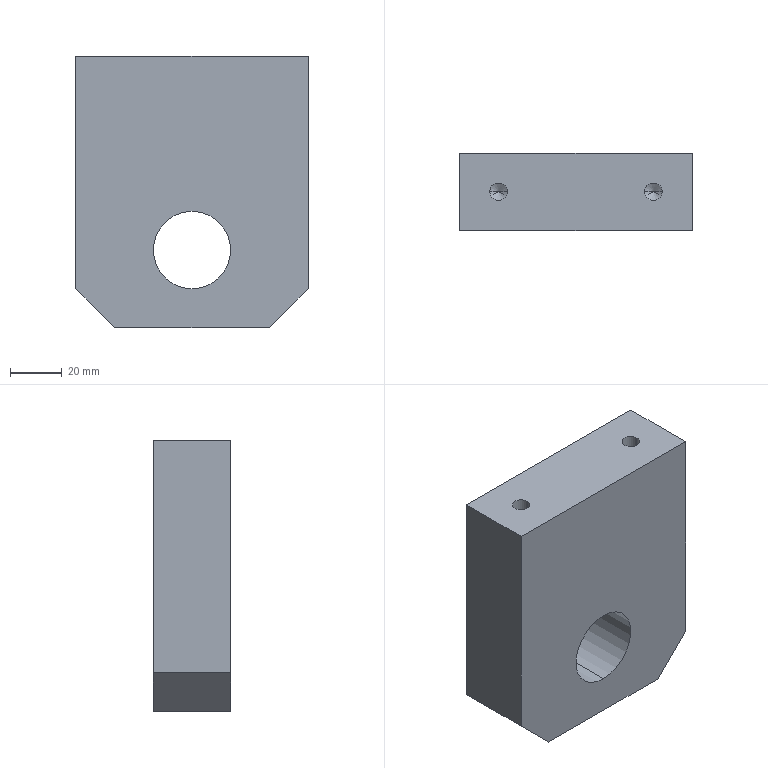Part | STEP file | PN_0020_default | 1 solid | 18 faces | box 90 x 30 x 105 mm | volume 254060 mm3 | plane 8 | cylinder 6 | cone 4 | commonest cylinder face diameters 6.8 x4 30 x2
STEP:
#1=CARTESIAN_POINT('',(0.,0.,0.));
#2=DIRECTION('',(0.,0.,1.));
#3=DIRECTION('',(1.,0.,0.));
#4=AXIS2_PLACEMENT_3D('',#1,#2,#3);
#5=CARTESIAN_POINT('',(-26.6,0.,32.75));
#6=VERTEX_POINT('',#5);
#7=CARTESIAN_POINT('',(-26.6,0.,52.5));
#8=VERTEX_POINT('',#7);
#9=CARTESIAN_POINT('',(-26.6,0.,52.5));
#10=DIRECTION('',(0.,0.,1.));
#11=VECTOR('',#10,1.);
#12=LINE('',#9,#11);
#13=CARTESIAN_POINT('',(-30.,0.,52.5));
#14=DIRECTION('',(0.,0.,1.));
#15=DIRECTION('',(1.,0.,0.));
#16=AXIS2_PLACEMENT_3D('',#13,#14,#15);
#17=CYLINDRICAL_SURFACE('',#16,3.4);
#18=CARTESIAN_POINT('',(6.283,0.));
#19=DIRECTION('',(0.,1.));
#20=VECTOR('',#19,1.);
#21=LINE('',#18,#20);
#22=(GEOMETRIC_REPRESENTATION_CONTEXT(2)PARAMETRIC_REPRESENTATION_CONTEXT()REPRESENTATION_CONTEXT('',''));
#23=DEFINITIONAL_REPRESENTATION('',(#21),#22);
#24=PCURVE('',#17,#23);
#25=CARTESIAN_POINT('',(-30.,0.,52.5));
#26=DIRECTION('',(0.,0.,1.));
#27=DIRECTION('',(1.,0.,0.));
#28=AXIS2_PLACEMENT_3D('',#25,#26,#27);
#29=CYLINDRICAL_SURFACE('',#28,3.4);
#30=CARTESIAN_POINT('',(0.,0.));
#31=DIRECTION('',(0.,1.));
#32=VECTOR('',#31,1.);
#33=LINE('',#30,#32);
#34=(GEOMETRIC_REPRESENTATION_CONTEXT(2)PARAMETRIC_REPRESENTATION_CONTEXT()REPRESENTATION_CONTEXT('',''));
#35=DEFINITIONAL_REPRESENTATION('',(#33),#34);
#36=PCURVE('',#29,#35);
#37=SURFACE_CURVE('',#12,(#24,#36),.PCURVE_S1.);
#38=EDGE_CURVE('',#6,#8,#37,.T.);
#39=ORIENTED_EDGE('',*,*,#38,.T.);
#40=CARTESIAN_POINT('',(-33.4,0.,52.5));
#41=VERTEX_POINT('',#40);
#42=CARTESIAN_POINT('',(-30.,0.,52.5));
#43=DIRECTION('',(0.,0.,1.));
#44=DIRECTION('',(1.,0.,0.));
#45=AXIS2_PLACEMENT_3D('',#42,#43,#44);
#46=CIRCLE('',#45,3.4);
#47=CARTESIAN_POINT('',(0.,0.));
#48=DIRECTION('',(1.,0.));
#49=VECTOR('',#48,1.);
#50=LINE('',#47,#49);
#51=(GEOMETRIC_REPRESENTATION_CONTEXT(2)PARAMETRIC_REPRESENTATION_CONTEXT()REPRESENTATION_CONTEXT('',''));
#52=DEFINITIONAL_REPRESENTATION('',(#50),#51);
#53=PCURVE('',#17,#52);
#54=CARTESIAN_POINT('',(45.,15.,52.5));
#55=DIRECTION('',(0.,0.,-1.));
#56=DIRECTION('',(-1.,0.,0.));
#57=AXIS2_PLACEMENT_3D('',#54,#55,#56);
#58=PLANE('',#57);
#59=CARTESIAN_POINT('',(71.6,-15.));
#60=CARTESIAN_POINT('',(71.6,-9.111));
#61=CARTESIAN_POINT('',(76.7,-12.056));
#62=CARTESIAN_POINT('',(81.8,-15.));
#63=CARTESIAN_POINT('',(76.7,-17.944));
#64=CARTESIAN_POINT('',(71.6,-20.889));
#65=CARTESIAN_POINT('',(71.6,-15.));
#66=(BOUNDED_CURVE()B_SPLINE_CURVE(2,(#59,#60,#61,#62,#63,#64,#65),.UNSPECIFIED.,.T.,.F.)B_SPLINE_CURVE_WITH_KNOTS((1,2,2,2,2,1),(-2.094,0.,2.094,4.189,6.283,8.378),.UNSPECIFIED.)CURVE()GEOMETRIC_REPRESENTATION_ITEM()RATIONAL_B_SPLINE_CURVE((1.,0.5,1.,0.5,1.,0.5,1.))REPRESENTATION_ITEM(''));
#67=(GEOMETRIC_REPRESENTATION_CONTEXT(2)PARAMETRIC_REPRESENTATION_CONTEXT()REPRESENTATION_CONTEXT('',''));
#68=DEFINITIONAL_REPRESENTATION('',(#66),#67);
#69=PCURVE('',#58,#68);
#70=SURFACE_CURVE('',#46,(#53,#69),.PCURVE_S1.);
#71=EDGE_CURVE('',#41,#8,#70,.T.);
#72=ORIENTED_EDGE('',*,*,#71,.F.);
#73=CARTESIAN_POINT('',(-33.4,0.,32.75));
#74=VERTEX_POINT('',#73);
#75=CARTESIAN_POINT('',(-33.4,0.,52.5));
#76=DIRECTION('',(0.,0.,1.));
#77=VECTOR('',#76,1.);
#78=LINE('',#75,#77);
#79=CARTESIAN_POINT('',(3.142,0.));
#80=DIRECTION('',(0.,1.));
#81=VECTOR('',#80,1.);
#82=LINE('',#79,#81);
#83=(GEOMETRIC_REPRESENTATION_CONTEXT(2)PARAMETRIC_REPRESENTATION_CONTEXT()REPRESENTATION_CONTEXT('',''));
#84=DEFINITIONAL_REPRESENTATION('',(#82),#83);
#85=PCURVE('',#17,#84);
#86=CARTESIAN_POINT('',(3.142,0.));
#87=DIRECTION('',(0.,1.));
#88=VECTOR('',#87,1.);
#89=LINE('',#86,#88);
#90=(GEOMETRIC_REPRESENTATION_CONTEXT(2)PARAMETRIC_REPRESENTATION_CONTEXT()REPRESENTATION_CONTEXT('',''));
#91=DEFINITIONAL_REPRESENTATION('',(#89),#90);
#92=PCURVE('',#29,#91);
#93=SURFACE_CURVE('',#78,(#85,#92),.PCURVE_S1.);
#94=EDGE_CURVE('',#74,#41,#93,.T.);
#95=ORIENTED_EDGE('',*,*,#94,.F.);
#96=CARTESIAN_POINT('',(-30.,0.,32.75));
#97=DIRECTION('',(0.,0.,1.));
#98=DIRECTION('',(1.,0.,0.));
#99=AXIS2_PLACEMENT_3D('',#96,#97,#98);
#100=CIRCLE('',#99,3.4);
#101=CARTESIAN_POINT('',(0.,-19.75));
#102=DIRECTION('',(1.,0.));
#103=VECTOR('',#102,1.);
#104=LINE('',#101,#103);
#105=(GEOMETRIC_REPRESENTATION_CONTEXT(2)PARAMETRIC_REPRESENTATION_CONTEXT()REPRESENTATION_CONTEXT('',''));
#106=DEFINITIONAL_REPRESENTATION('',(#104),#105);
#107=PCURVE('',#17,#106);
#108=CARTESIAN_POINT('',(-30.,0.,32.75));
#109=DIRECTION('',(0.,0.,1.));
#110=DIRECTION('',(1.,0.,0.));
#111=AXIS2_PLACEMENT_3D('',#108,#109,#110);
#112=CONICAL_SURFACE('',#111,3.4,1.03);
#113=CARTESIAN_POINT('',(0.,0.));
#114=DIRECTION('',(1.,0.));
#115=VECTOR('',#114,1.);
#116=LINE('',#113,#115);
#117=(GEOMETRIC_REPRESENTATION_CONTEXT(2)PARAMETRIC_REPRESENTATION_CONTEXT()REPRESENTATION_CONTEXT('',''));
#118=DEFINITIONAL_REPRESENTATION('',(#116),#117);
#119=PCURVE('',#112,#118);
#120=SURFACE_CURVE('',#100,(#107,#119),.PCURVE_S1.);
#121=EDGE_CURVE('',#74,#6,#120,.T.);
#122=ORIENTED_EDGE('',*,*,#121,.T.);
#123=EDGE_LOOP('',(#39,#72,#95,#122));
#124=FACE_BOUND('',#123,.F.);
#125=ADVANCED_FACE('',(#124),#17,.F.);
#126=ORIENTED_EDGE('',*,*,#121,.F.);
#127=CARTESIAN_POINT('',(-30.,0.,30.707));
#128=VERTEX_POINT('',#127);
#129=CARTESIAN_POINT('',(-33.4,0.,32.75));
#130=DIRECTION('',(-0.8572,0.,0.515));
#131=VECTOR('',#130,1.);
#132=LINE('',#129,#131);
#133=CARTESIAN_POINT('',(3.142,0.));
#134=DIRECTION('',(0.,1.));
#135=VECTOR('',#134,1.);
#136=LINE('',#133,#135);
#137=(GEOMETRIC_REPRESENTATION_CONTEXT(2)PARAMETRIC_REPRESENTATION_CONTEXT()REPRESENTATION_CONTEXT('',''));
#138=DEFINITIONAL_REPRESENTATION('',(#136),#137);
#139=PCURVE('',#112,#138);
#140=CARTESIAN_POINT('',(-30.,0.,32.75));
#141=DIRECTION('',(0.,0.,1.));
#142=DIRECTION('',(1.,0.,0.));
#143=AXIS2_PLACEMENT_3D('',#140,#141,#142);
#144=CONICAL_SURFACE('',#143,3.4,1.03);
#145=CARTESIAN_POINT('',(3.142,0.));
#146=DIRECTION('',(0.,1.));
#147=VECTOR('',#146,1.);
#148=LINE('',#145,#147);
#149=(GEOMETRIC_REPRESENTATION_CONTEXT(2)PARAMETRIC_REPRESENTATION_CONTEXT()REPRESENTATION_CONTEXT('',''));
#150=DEFINITIONAL_REPRESENTATION('',(#148),#149);
#151=PCURVE('',#144,#150);
#152=SURFACE_CURVE('',#132,(#139,#151),.PCURVE_S1.);
#153=EDGE_CURVE('',#128,#74,#152,.T.);
#154=ORIENTED_EDGE('',*,*,#153,.F.);
#155=CARTESIAN_POINT('',(-26.6,0.,32.75));
#156=DIRECTION('',(0.8572,0.,0.515));
#157=VECTOR('',#156,1.);
#158=LINE('',#155,#157);
#159=CARTESIAN_POINT('',(6.283,0.));
#160=DIRECTION('',(0.,1.));
#161=VECTOR('',#160,1.);
#162=LINE('',#159,#161);
#163=(GEOMETRIC_REPRESENTATION_CONTEXT(2)PARAMETRIC_REPRESENTATION_CONTEXT()REPRESENTATION_CONTEXT('',''));
#164=DEFINITIONAL_REPRESENTATION('',(#162),#163);
#165=PCURVE('',#112,#164);
#166=CARTESIAN_POINT('',(0.,0.));
#167=DIRECTION('',(0.,1.));
#168=VECTOR('',#167,1.);
#169=LINE('',#166,#168);
#170=(GEOMETRIC_REPRESENTATION_CONTEXT(2)PARAMETRIC_REPRESENTATION_CONTEXT()REPRESENTATION_CONTEXT('',''));
#171=DEFINITIONAL_REPRESENTATION('',(#169),#170);
#172=PCURVE('',#144,#171);
#173=SURFACE_CURVE('',#158,(#165,#172),.PCURVE_S1.);
#174=EDGE_CURVE('',#128,#6,#173,.T.);
#175=ORIENTED_EDGE('',*,*,#174,.T.);
#176=EDGE_LOOP('',(#126,#154,#175));
#177=FACE_BOUND('',#176,.F.);
#178=ADVANCED_FACE('',(#177),#112,.F.);
#179=CARTESIAN_POINT('',(33.4,0.,32.75));
#180=VERTEX_POINT('',#179);
#181=CARTESIAN_POINT('',(33.4,0.,52.5));
#182=VERTEX_POINT('',#181);
#183=CARTESIAN_POINT('',(33.4,0.,52.5));
#184=DIRECTION('',(0.,0.,1.));
#185=VECTOR('',#184,1.);
#186=LINE('',#183,#185);
#187=CARTESIAN_POINT('',(30.,0.,52.5));
#188=DIRECTION('',(0.,0.,1.));
#189=DIRECTION('',(1.,0.,0.));
#190=AXIS2_PLACEMENT_3D('',#187,#188,#189);
#191=CYLINDRICAL_SURFACE('',#190,3.4);
#192=CARTESIAN_POINT('',(6.283,0.));
#193=DIRECTION('',(0.,1.));
#194=VECTOR('',#193,1.);
#195=LINE('',#192,#194);
#196=(GEOMETRIC_REPRESENTATION_CONTEXT(2)PARAMETRIC_REPRESENTATION_CONTEXT()REPRESENTATION_CONTEXT('',''));
#197=DEFINITIONAL_REPRESENTATION('',(#195),#196);
#198=PCURVE('',#191,#197);
#199=CARTESIAN_POINT('',(30.,0.,52.5));
#200=DIRECTION('',(0.,0.,1.));
#201=DIRECTION('',(1.,0.,0.));
#202=AXIS2_PLACEMENT_3D('',#199,#200,#201);
#203=CYLINDRICAL_SURFACE('',#202,3.4);
#204=CARTESIAN_POINT('',(0.,0.));
#205=DIRECTION('',(0.,1.));
#206=VECTOR('',#205,1.);
#207=LINE('',#204,#206);
#208=(GEOMETRIC_REPRESENTATION_CONTEXT(2)PARAMETRIC_REPRESENTATION_CONTEXT()REPRESENTATION_CONTEXT('',''));
#209=DEFINITIONAL_REPRESENTATION('',(#207),#208);
#210=PCURVE('',#203,#209);
#211=SURFACE_CURVE('',#186,(#198,#210),.PCURVE_S1.);
#212=EDGE_CURVE('',#180,#182,#211,.T.);
#213=ORIENTED_EDGE('',*,*,#212,.T.);
#214=CARTESIAN_POINT('',(26.6,0.,52.5));
#215=VERTEX_POINT('',#214);
#216=CARTESIAN_POINT('',(30.,0.,52.5));
#217=DIRECTION('',(0.,0.,1.));
#218=DIRECTION('',(1.,0.,0.));
#219=AXIS2_PLACEMENT_3D('',#216,#217,#218);
#220=CIRCLE('',#219,3.4);
#221=CARTESIAN_POINT('',(0.,0.));
#222=DIRECTION('',(1.,0.));
#223=VECTOR('',#222,1.);
#224=LINE('',#221,#223);
#225=(GEOMETRIC_REPRESENTATION_CONTEXT(2)PARAMETRIC_REPRESENTATION_CONTEXT()REPRESENTATION_CONTEXT('',''));
#226=DEFINITIONAL_REPRESENTATION('',(#224),#225);
#227=PCURVE('',#191,#226);
#228=CARTESIAN_POINT('',(11.6,-15.));
#229=CARTESIAN_POINT('',(11.6,-9.111));
#230=CARTESIAN_POINT('',(16.7,-12.056));
#231=CARTESIAN_POINT('',(21.8,-15.));
#232=CARTESIAN_POINT('',(16.7,-17.944));
#233=CARTESIAN_POINT('',(11.6,-20.889));
#234=CARTESIAN_POINT('',(11.6,-15.));
#235=(BOUNDED_CURVE()B_SPLINE_CURVE(2,(#228,#229,#230,#231,#232,#233,#234),.UNSPECIFIED.,.T.,.F.)B_SPLINE_CURVE_WITH_KNOTS((1,2,2,2,2,1),(-2.094,0.,2.094,4.189,6.283,8.378),.UNSPECIFIED.)CURVE()GEOMETRIC_REPRESENTATION_ITEM()RATIONAL_B_SPLINE_CURVE((1.,0.5,1.,0.5,1.,0.5,1.))REPRESENTATION_ITEM(''));
#236=(GEOMETRIC_REPRESENTATION_CONTEXT(2)PARAMETRIC_REPRESENTATION_CONTEXT()REPRESENTATION_CONTEXT('',''));
#237=DEFINITIONAL_REPRESENTATION('',(#235),#236);
#238=PCURVE('',#58,#237);
#239=SURFACE_CURVE('',#220,(#227,#238),.PCURVE_S1.);
#240=EDGE_CURVE('',#215,#182,#239,.T.);
#241=ORIENTED_EDGE('',*,*,#240,.F.);
#242=CARTESIAN_POINT('',(26.6,0.,32.75));
#243=VERTEX_POINT('',#242);
#244=CARTESIAN_POINT('',(26.6,0.,52.5));
#245=DIRECTION('',(0.,0.,1.));
#246=VECTOR('',#245,1.);
#247=LINE('',#244,#246);
#248=CARTESIAN_POINT('',(3.142,0.));
#249=DIRECTION('',(0.,1.));
#250=VECTOR('',#249,1.);
#251=LINE('',#248,#250);
#252=(GEOMETRIC_REPRESENTATION_CONTEXT(2)PARAMETRIC_REPRESENTATION_CONTEXT()REPRESENTATION_CONTEXT('',''));
#253=DEFINITIONAL_REPRESENTATION('',(#251),#252);
#254=PCURVE('',#191,#253);
#255=CARTESIAN_POINT('',(3.142,0.));
#256=DIRECTION('',(0.,1.));
#257=VECTOR('',#256,1.);
#258=LINE('',#255,#257);
#259=(GEOMETRIC_REPRESENTATION_CONTEXT(2)PARAMETRIC_REPRESENTATION_CONTEXT()REPRESENTATION_CONTEXT('',''));
#260=DEFINITIONAL_REPRESENTATION('',(#258),#259);
#261=PCURVE('',#203,#260);
#262=SURFACE_CURVE('',#247,(#254,#261),.PCURVE_S1.);
#263=EDGE_CURVE('',#243,#215,#262,.T.);
#264=ORIENTED_EDGE('',*,*,#263,.F.);
#265=CARTESIAN_POINT('',(30.,0.,32.75));
#266=DIRECTION('',(0.,0.,1.));
#267=DIRECTION('',(1.,0.,0.));
#268=AXIS2_PLACEMENT_3D('',#265,#266,#267);
#269=CIRCLE('',#268,3.4);
#270=CARTESIAN_POINT('',(0.,-19.75));
#271=DIRECTION('',(1.,0.));
#272=VECTOR('',#271,1.);
#273=LINE('',#270,#272);
#274=(GEOMETRIC_REPRESENTATION_CONTEXT(2)PARAMETRIC_REPRESENTATION_CONTEXT()REPRESENTATION_CONTEXT('',''));
#275=DEFINITIONAL_REPRESENTATION('',(#273),#274);
#276=PCURVE('',#191,#275);
#277=CARTESIAN_POINT('',(30.,0.,32.75));
#278=DIRECTION('',(0.,0.,1.));
#279=DIRECTION('',(1.,0.,0.));
#280=AXIS2_PLACEMENT_3D('',#277,#278,#279);
#281=CONICAL_SURFACE('',#280,3.4,1.03);
#282=CARTESIAN_POINT('',(0.,0.));
#283=DIRECTION('',(1.,0.));
#284=VECTOR('',#283,1.);
#285=LINE('',#282,#284);
#286=(GEOMETRIC_REPRESENTATION_CONTEXT(2)PARAMETRIC_REPRESENTATION_CONTEXT()REPRESENTATION_CONTEXT('',''));
#287=DEFINITIONAL_REPRESENTATION('',(#285),#286);
#288=PCURVE('',#281,#287);
#289=SURFACE_CURVE('',#269,(#276,#288),.PCURVE_S1.);
#290=EDGE_CURVE('',#243,#180,#289,.T.);
#291=ORIENTED_EDGE('',*,*,#290,.T.);
#292=EDGE_LOOP('',(#213,#241,#264,#291));
#293=FACE_BOUND('',#292,.F.);
#294=ADVANCED_FACE('',(#293),#191,.F.);
#295=ORIENTED_EDGE('',*,*,#290,.F.);
#296=CARTESIAN_POINT('',(30.,0.,30.707));
#297=VERTEX_POINT('',#296);
#298=CARTESIAN_POINT('',(26.6,0.,32.75));
#299=DIRECTION('',(-0.8572,0.,0.515));
#300=VECTOR('',#299,1.);
#301=LINE('',#298,#300);
#302=CARTESIAN_POINT('',(3.142,0.));
#303=DIRECTION('',(0.,1.));
#304=VECTOR('',#303,1.);
#305=LINE('',#302,#304);
#306=(GEOMETRIC_REPRESENTATION_CONTEXT(2)PARAMETRIC_REPRESENTATION_CONTEXT()REPRESENTATION_CONTEXT('',''));
#307=DEFINITIONAL_REPRESENTATION('',(#305),#306);
#308=PCURVE('',#281,#307);
#309=CARTESIAN_POINT('',(30.,0.,32.75));
#310=DIRECTION('',(0.,0.,1.));
#311=DIRECTION('',(1.,0.,0.));
#312=AXIS2_PLACEMENT_3D('',#309,#310,#311);
#313=CONICAL_SURFACE('',#312,3.4,1.03);
#314=CARTESIAN_POINT('',(3.142,0.));
#315=DIRECTION('',(0.,1.));
#316=VECTOR('',#315,1.);
#317=LINE('',#314,#316);
#318=(GEOMETRIC_REPRESENTATION_CONTEXT(2)PARAMETRIC_REPRESENTATION_CONTEXT()REPRESENTATION_CONTEXT('',''));
#319=DEFINITIONAL_REPRESENTATION('',(#317),#318);
#320=PCURVE('',#313,#319);
#321=SURFACE_CURVE('',#301,(#308,#320),.PCURVE_S1.);
#322=EDGE_CURVE('',#297,#243,#321,.T.);
#323=ORIENTED_EDGE('',*,*,#322,.F.);
#324=CARTESIAN_POINT('',(33.4,0.,32.75));
#325=DIRECTION('',(0.8572,0.,0.515));
#326=VECTOR('',#325,1.);
#327=LINE('',#324,#326);
#328=CARTESIAN_POINT('',(6.283,0.));
#329=DIRECTION('',(0.,1.));
#330=VECTOR('',#329,1.);
#331=LINE('',#328,#330);
#332=(GEOMETRIC_REPRESENTATION_CONTEXT(2)PARAMETRIC_REPRESENTATION_CONTEXT()REPRESENTATION_CONTEXT('',''));
#333=DEFINITIONAL_REPRESENTATION('',(#331),#332);
#334=PCURVE('',#281,#333);
#335=CARTESIAN_POINT('',(0.,0.));
#336=DIRECTION('',(0.,1.));
#337=VECTOR('',#336,1.);
#338=LINE('',#335,#337);
#339=(GEOMETRIC_REPRESENTATION_CONTEXT(2)PARAMETRIC_REPRESENTATION_CONTEXT()REPRESENTATION_CONTEXT('',''));
#340=DEFINITIONAL_REPRESENTATION('',(#338),#339);
#341=PCURVE('',#313,#340);
#342=SURFACE_CURVE('',#327,(#334,#341),.PCURVE_S1.);
#343=EDGE_CURVE('',#297,#180,#342,.T.);
#344=ORIENTED_EDGE('',*,*,#343,.T.);
#345=EDGE_LOOP('',(#295,#323,#344));
#346=FACE_BOUND('',#345,.F.);
#347=ADVANCED_FACE('',(#346),#281,.F.);
#348=CARTESIAN_POINT('',(0.,-15.,-7.5));
#349=VERTEX_POINT('',#348);
#350=CARTESIAN_POINT('',(0.,15.,-7.5));
#351=VERTEX_POINT('',#350);
#352=CARTESIAN_POINT('',(0.,-15.,-7.5));
#353=DIRECTION('',(0.,1.,0.));
#354=VECTOR('',#353,1.);
#355=LINE('',#352,#354);
#356=CARTESIAN_POINT('',(0.,-15.,-22.5));
#357=DIRECTION('',(0.,1.,0.));
#358=DIRECTION('',(0.,0.,1.));
#359=AXIS2_PLACEMENT_3D('',#356,#357,#358);
#360=CYLINDRICAL_SURFACE('',#359,15.);
#361=CARTESIAN_POINT('',(6.283,0.));
#362=DIRECTION('',(0.,1.));
#363=VECTOR('',#362,1.);
#364=LINE('',#361,#363);
#365=(GEOMETRIC_REPRESENTATION_CONTEXT(2)PARAMETRIC_REPRESENTATION_CONTEXT()REPRESENTATION_CONTEXT('',''));
#366=DEFINITIONAL_REPRESENTATION('',(#364),#365);
#367=PCURVE('',#360,#366);
#368=CARTESIAN_POINT('',(0.,-15.,-22.5));
#369=DIRECTION('',(0.,1.,0.));
#370=DIRECTION('',(0.,0.,1.));
#371=AXIS2_PLACEMENT_3D('',#368,#369,#370);
#372=CYLINDRICAL_SURFACE('',#371,15.);
#373=CARTESIAN_POINT('',(0.,0.));
#374=DIRECTION('',(0.,1.));
#375=VECTOR('',#374,1.);
#376=LINE('',#373,#375);
#377=(GEOMETRIC_REPRESENTATION_CONTEXT(2)PARAMETRIC_REPRESENTATION_CONTEXT()REPRESENTATION_CONTEXT('',''));
#378=DEFINITIONAL_REPRESENTATION('',(#376),#377);
#379=PCURVE('',#372,#378);
#380=SURFACE_CURVE('',#355,(#367,#379),.PCURVE_S1.);
#381=EDGE_CURVE('',#349,#351,#380,.T.);
#382=ORIENTED_EDGE('',*,*,#381,.T.);
#383=CARTESIAN_POINT('',(0.,15.,-37.5));
#384=VERTEX_POINT('',#383);
#385=CARTESIAN_POINT('',(0.,15.,-22.5));
#386=DIRECTION('',(0.,1.,0.));
#387=DIRECTION('',(0.,0.,1.));
#388=AXIS2_PLACEMENT_3D('',#385,#386,#387);
#389=CIRCLE('',#388,15.);
#390=CARTESIAN_POINT('',(0.,30.));
#391=DIRECTION('',(1.,0.));
#392=VECTOR('',#391,1.);
#393=LINE('',#390,#392);
#394=(GEOMETRIC_REPRESENTATION_CONTEXT(2)PARAMETRIC_REPRESENTATION_CONTEXT()REPRESENTATION_CONTEXT('',''));
#395=DEFINITIONAL_REPRESENTATION('',(#393),#394);
#396=PCURVE('',#360,#395);
#397=CARTESIAN_POINT('',(-45.,15.,-52.5));
#398=DIRECTION('',(0.,1.,0.));
#399=DIRECTION('',(0.,0.,1.));
#400=AXIS2_PLACEMENT_3D('',#397,#398,#399);
#401=PLANE('',#400);
#402=CARTESIAN_POINT('',(30.,45.));
#403=DIRECTION('',(1.,0.));
#404=AXIS2_PLACEMENT_2D('',#402,#403);
#405=CIRCLE('',#404,15.);
#406=(GEOMETRIC_REPRESENTATION_CONTEXT(2)PARAMETRIC_REPRESENTATION_CONTEXT()REPRESENTATION_CONTEXT('',''));
#407=DEFINITIONAL_REPRESENTATION('',(#405),#406);
#408=PCURVE('',#401,#407);
#409=SURFACE_CURVE('',#389,(#396,#408),.PCURVE_S1.);
#410=EDGE_CURVE('',#384,#351,#409,.T.);
#411=ORIENTED_EDGE('',*,*,#410,.F.);
#412=CARTESIAN_POINT('',(0.,-15.,-37.5));
#413=VERTEX_POINT('',#412);
#414=CARTESIAN_POINT('',(0.,-15.,-37.5));
#415=DIRECTION('',(0.,1.,0.));
#416=VECTOR('',#415,1.);
#417=LINE('',#414,#416);
#418=CARTESIAN_POINT('',(3.142,0.));
#419=DIRECTION('',(0.,1.));
#420=VECTOR('',#419,1.);
#421=LINE('',#418,#420);
#422=(GEOMETRIC_REPRESENTATION_CONTEXT(2)PARAMETRIC_REPRESENTATION_CONTEXT()REPRESENTATION_CONTEXT('',''));
#423=DEFINITIONAL_REPRESENTATION('',(#421),#422);
#424=PCURVE('',#360,#423);
#425=CARTESIAN_POINT('',(3.142,0.));
#426=DIRECTION('',(0.,1.));
#427=VECTOR('',#426,1.);
#428=LINE('',#425,#427);
#429=(GEOMETRIC_REPRESENTATION_CONTEXT(2)PARAMETRIC_REPRESENTATION_CONTEXT()REPRESENTATION_CONTEXT('',''));
#430=DEFINITIONAL_REPRESENTATION('',(#428),#429);
#431=PCURVE('',#372,#430);
#432=SURFACE_CURVE('',#417,(#424,#431),.PCURVE_S1.);
#433=EDGE_CURVE('',#413,#384,#432,.T.);
#434=ORIENTED_EDGE('',*,*,#433,.F.);
#435=CARTESIAN_POINT('',(0.,-15.,-22.5));
#436=DIRECTION('',(0.,1.,0.));
#437=DIRECTION('',(0.,0.,1.));
#438=AXIS2_PLACEMENT_3D('',#435,#436,#437);
#439=CIRCLE('',#438,15.);
#440=CARTESIAN_POINT('',(0.,0.));
#441=DIRECTION('',(1.,0.));
#442=VECTOR('',#441,1.);
#443=LINE('',#440,#442);
#444=(GEOMETRIC_REPRESENTATION_CONTEXT(2)PARAMETRIC_REPRESENTATION_CONTEXT()REPRESENTATION_CONTEXT('',''));
#445=DEFINITIONAL_REPRESENTATION('',(#443),#444);
#446=PCURVE('',#360,#445);
#447=CARTESIAN_POINT('',(-45.,-15.,-52.5));
#448=DIRECTION('',(0.,1.,0.));
#449=DIRECTION('',(0.,0.,1.));
#450=AXIS2_PLACEMENT_3D('',#447,#448,#449);
#451=PLANE('',#450);
#452=CARTESIAN_POINT('',(30.,45.));
#453=DIRECTION('',(1.,0.));
#454=AXIS2_PLACEMENT_2D('',#452,#453);
#455=CIRCLE('',#454,15.);
#456=(GEOMETRIC_REPRESENTATION_CONTEXT(2)PARAMETRIC_REPRESENTATION_CONTEXT()REPRESENTATION_CONTEXT('',''));
#457=DEFINITIONAL_REPRESENTATION('',(#455),#456);
#458=PCURVE('',#451,#457);
#459=SURFACE_CURVE('',#439,(#446,#458),.PCURVE_S1.);
#460=EDGE_CURVE('',#413,#349,#459,.T.);
#461=ORIENTED_EDGE('',*,*,#460,.T.);
#462=EDGE_LOOP('',(#382,#411,#434,#461));
#463=FACE_BOUND('',#462,.F.);
#464=ADVANCED_FACE('',(#463),#360,.F.);
#465=CARTESIAN_POINT('',(-45.,15.,-37.5));
#466=VERTEX_POINT('',#465);
#467=CARTESIAN_POINT('',(-45.,15.,52.5));
#468=VERTEX_POINT('',#467);
#469=CARTESIAN_POINT('',(-45.,15.,52.5));
#470=DIRECTION('',(0.,0.,1.));
#471=VECTOR('',#470,1.);
#472=LINE('',#469,#471);
#473=CARTESIAN_POINT('',(-45.,15.,52.5));
#474=DIRECTION('',(1.,0.,0.));
#475=DIRECTION('',(0.,0.,-1.));
#476=AXIS2_PLACEMENT_3D('',#473,#474,#475);
#477=PLANE('',#476);
#478=CARTESIAN_POINT('',(0.,0.));
#479=DIRECTION('',(-1.,0.));
#480=VECTOR('',#479,1.);
#481=LINE('',#478,#480);
#482=(GEOMETRIC_REPRESENTATION_CONTEXT(2)PARAMETRIC_REPRESENTATION_CONTEXT()REPRESENTATION_CONTEXT('',''));
#483=DEFINITIONAL_REPRESENTATION('',(#481),#482);
#484=PCURVE('',#477,#483);
#485=CARTESIAN_POINT('',(105.,0.));
#486=DIRECTION('',(1.,0.));
#487=VECTOR('',#486,1.);
#488=LINE('',#485,#487);
#489=(GEOMETRIC_REPRESENTATION_CONTEXT(2)PARAMETRIC_REPRESENTATION_CONTEXT()REPRESENTATION_CONTEXT('',''));
#490=DEFINITIONAL_REPRESENTATION('',(#488),#489);
#491=PCURVE('',#401,#490);
#492=SURFACE_CURVE('',#472,(#484,#491),.PCURVE_S1.);
#493=EDGE_CURVE('',#466,#468,#492,.T.);
#494=ORIENTED_EDGE('',*,*,#493,.F.);
#495=CARTESIAN_POINT('',(-45.,-15.,-37.5));
#496=VERTEX_POINT('',#495);
#497=CARTESIAN_POINT('',(-45.,15.,-37.5));
#498=DIRECTION('',(0.,-1.,0.));
#499=VECTOR('',#498,1.);
#500=LINE('',#497,#499);
#501=CARTESIAN_POINT('',(90.,0.));
#502=DIRECTION('',(0.,-1.));
#503=VECTOR('',#502,1.);
#504=LINE('',#501,#503);
#505=(GEOMETRIC_REPRESENTATION_CONTEXT(2)PARAMETRIC_REPRESENTATION_CONTEXT()REPRESENTATION_CONTEXT('',''));
#506=DEFINITIONAL_REPRESENTATION('',(#504),#505);
#507=PCURVE('',#477,#506);
#508=CARTESIAN_POINT('',(-45.,15.,-37.5));
#509=DIRECTION('',(0.7071,0.,0.7071));
#510=DIRECTION('',(0.7071,0.,-0.7071));
#511=AXIS2_PLACEMENT_3D('',#508,#509,#510);
#512=PLANE('',#511);
#513=CARTESIAN_POINT('',(0.,0.));
#514=DIRECTION('',(0.,-1.));
#515=VECTOR('',#514,1.);
#516=LINE('',#513,#515);
#517=(GEOMETRIC_REPRESENTATION_CONTEXT(2)PARAMETRIC_REPRESENTATION_CONTEXT()REPRESENTATION_CONTEXT('',''));
#518=DEFINITIONAL_REPRESENTATION('',(#516),#517);
#519=PCURVE('',#512,#518);
#520=SURFACE_CURVE('',#500,(#507,#519),.PCURVE_S1.);
#521=EDGE_CURVE('',#466,#496,#520,.T.);
#522=ORIENTED_EDGE('',*,*,#521,.T.);
#523=CARTESIAN_POINT('',(-45.,-15.,52.5));
#524=VERTEX_POINT('',#523);
#525=CARTESIAN_POINT('',(-45.,-15.,52.5));
#526=DIRECTION('',(0.,0.,1.));
#527=VECTOR('',#526,1.);
#528=LINE('',#525,#527);
#529=CARTESIAN_POINT('',(0.,-30.));
#530=DIRECTION('',(-1.,0.));
#531=VECTOR('',#530,1.);
#532=LINE('',#529,#531);
#533=(GEOMETRIC_REPRESENTATION_CONTEXT(2)PARAMETRIC_REPRESENTATION_CONTEXT()REPRESENTATION_CONTEXT('',''));
#534=DEFINITIONAL_REPRESENTATION('',(#532),#533);
#535=PCURVE('',#477,#534);
#536=CARTESIAN_POINT('',(105.,0.));
#537=DIRECTION('',(1.,0.));
#538=VECTOR('',#537,1.);
#539=LINE('',#536,#538);
#540=(GEOMETRIC_REPRESENTATION_CONTEXT(2)PARAMETRIC_REPRESENTATION_CONTEXT()REPRESENTATION_CONTEXT('',''));
#541=DEFINITIONAL_REPRESENTATION('',(#539),#540);
#542=PCURVE('',#451,#541);
#543=SURFACE_CURVE('',#528,(#535,#542),.PCURVE_S1.);
#544=EDGE_CURVE('',#496,#524,#543,.T.);
#545=ORIENTED_EDGE('',*,*,#544,.T.);
#546=CARTESIAN_POINT('',(-45.,15.,52.5));
#547=DIRECTION('',(0.,-1.,0.));
#548=VECTOR('',#547,1.);
#549=LINE('',#546,#548);
#550=CARTESIAN_POINT('',(0.,0.));
#551=DIRECTION('',(0.,-1.));
#552=VECTOR('',#551,1.);
#553=LINE('',#550,#552);
#554=(GEOMETRIC_REPRESENTATION_CONTEXT(2)PARAMETRIC_REPRESENTATION_CONTEXT()REPRESENTATION_CONTEXT('',''));
#555=DEFINITIONAL_REPRESENTATION('',(#553),#554);
#556=PCURVE('',#477,#555);
#557=CARTESIAN_POINT('',(90.,0.));
#558=DIRECTION('',(0.,-1.));
#559=VECTOR('',#558,1.);
#560=LINE('',#557,#559);
#561=(GEOMETRIC_REPRESENTATION_CONTEXT(2)PARAMETRIC_REPRESENTATION_CONTEXT()REPRESENTATION_CONTEXT('',''));
#562=DEFINITIONAL_REPRESENTATION('',(#560),#561);
#563=PCURVE('',#58,#562);
#564=SURFACE_CURVE('',#549,(#556,#563),.PCURVE_S1.);
#565=EDGE_CURVE('',#468,#524,#564,.T.);
#566=ORIENTED_EDGE('',*,*,#565,.F.);
#567=EDGE_LOOP('',(#494,#522,#545,#566));
#568=FACE_BOUND('',#567,.T.);
#569=ADVANCED_FACE('',(#568),#477,.F.);
#570=CARTESIAN_POINT('',(-30.,0.,52.5));
#571=DIRECTION('',(0.,0.,1.));
#572=DIRECTION('',(1.,0.,0.));
#573=AXIS2_PLACEMENT_3D('',#570,#571,#572);
#574=CIRCLE('',#573,3.4);
#575=CARTESIAN_POINT('',(71.6,-15.));
#576=CARTESIAN_POINT('',(71.6,-9.111));
#577=CARTESIAN_POINT('',(76.7,-12.056));
#578=CARTESIAN_POINT('',(81.8,-15.));
#579=CARTESIAN_POINT('',(76.7,-17.944));
#580=CARTESIAN_POINT('',(71.6,-20.889));
#581=CARTESIAN_POINT('',(71.6,-15.));
#582=(BOUNDED_CURVE()B_SPLINE_CURVE(2,(#575,#576,#577,#578,#579,#580,#581),.UNSPECIFIED.,.T.,.F.)B_SPLINE_CURVE_WITH_KNOTS((1,2,2,2,2,1),(-2.094,0.,2.094,4.189,6.283,8.378),.UNSPECIFIED.)CURVE()GEOMETRIC_REPRESENTATION_ITEM()RATIONAL_B_SPLINE_CURVE((1.,0.5,1.,0.5,1.,0.5,1.))REPRESENTATION_ITEM(''));
#583=(GEOMETRIC_REPRESENTATION_CONTEXT(2)PARAMETRIC_REPRESENTATION_CONTEXT()REPRESENTATION_CONTEXT('',''));
#584=DEFINITIONAL_REPRESENTATION('',(#582),#583);
#585=PCURVE('',#58,#584);
#586=CARTESIAN_POINT('',(0.,0.));
#587=DIRECTION('',(1.,0.));
#588=VECTOR('',#587,1.);
#589=LINE('',#586,#588);
#590=(GEOMETRIC_REPRESENTATION_CONTEXT(2)PARAMETRIC_REPRESENTATION_CONTEXT()REPRESENTATION_CONTEXT('',''));
#591=DEFINITIONAL_REPRESENTATION('',(#589),#590);
#592=PCURVE('',#29,#591);
#593=SURFACE_CURVE('',#574,(#585,#592),.PCURVE_S1.);
#594=EDGE_CURVE('',#8,#41,#593,.T.);
#595=ORIENTED_EDGE('',*,*,#594,.F.);
#596=ORIENTED_EDGE('',*,*,#71,.F.);
#597=EDGE_LOOP('',(#595,#596));
#598=FACE_BOUND('',#597,.T.);
#599=CARTESIAN_POINT('',(30.,0.,52.5));
#600=DIRECTION('',(0.,0.,1.));
#601=DIRECTION('',(1.,0.,0.));
#602=AXIS2_PLACEMENT_3D('',#599,#600,#601);
#603=CIRCLE('',#602,3.4);
#604=CARTESIAN_POINT('',(11.6,-15.));
#605=CARTESIAN_POINT('',(11.6,-9.111));
#606=CARTESIAN_POINT('',(16.7,-12.056));
#607=CARTESIAN_POINT('',(21.8,-15.));
#608=CARTESIAN_POINT('',(16.7,-17.944));
#609=CARTESIAN_POINT('',(11.6,-20.889));
#610=CARTESIAN_POINT('',(11.6,-15.));
#611=(BOUNDED_CURVE()B_SPLINE_CURVE(2,(#604,#605,#606,#607,#608,#609,#610),.UNSPECIFIED.,.T.,.F.)B_SPLINE_CURVE_WITH_KNOTS((1,2,2,2,2,1),(-2.094,0.,2.094,4.189,6.283,8.378),.UNSPECIFIED.)CURVE()GEOMETRIC_REPRESENTATION_ITEM()RATIONAL_B_SPLINE_CURVE((1.,0.5,1.,0.5,1.,0.5,1.))REPRESENTATION_ITEM(''));
#612=(GEOMETRIC_REPRESENTATION_CONTEXT(2)PARAMETRIC_REPRESENTATION_CONTEXT()REPRESENTATION_CONTEXT('',''));
#613=DEFINITIONAL_REPRESENTATION('',(#611),#612);
#614=PCURVE('',#58,#613);
#615=CARTESIAN_POINT('',(0.,0.));
#616=DIRECTION('',(1.,0.));
#617=VECTOR('',#616,1.);
#618=LINE('',#615,#617);
#619=(GEOMETRIC_REPRESENTATION_CONTEXT(2)PARAMETRIC_REPRESENTATION_CONTEXT()REPRESENTATION_CONTEXT('',''));
#620=DEFINITIONAL_REPRESENTATION('',(#618),#619);
#621=PCURVE('',#203,#620);
#622=SURFACE_CURVE('',#603,(#614,#621),.PCURVE_S1.);
#623=EDGE_CURVE('',#182,#215,#622,.T.);
#624=ORIENTED_EDGE('',*,*,#623,.F.);
#625=ORIENTED_EDGE('',*,*,#240,.F.);
#626=EDGE_LOOP('',(#624,#625));
#627=FACE_BOUND('',#626,.T.);
#628=CARTESIAN_POINT('',(45.,-15.,52.5));
#629=VERTEX_POINT('',#628);
#630=CARTESIAN_POINT('',(45.,-15.,52.5));
#631=DIRECTION('',(1.,0.,0.));
#632=VECTOR('',#631,1.);
#633=LINE('',#630,#632);
#634=CARTESIAN_POINT('',(0.,-30.));
#635=DIRECTION('',(-1.,0.));
#636=VECTOR('',#635,1.);
#637=LINE('',#634,#636);
#638=(GEOMETRIC_REPRESENTATION_CONTEXT(2)PARAMETRIC_REPRESENTATION_CONTEXT()REPRESENTATION_CONTEXT('',''));
#639=DEFINITIONAL_REPRESENTATION('',(#637),#638);
#640=PCURVE('',#58,#639);
#641=CARTESIAN_POINT('',(105.,90.));
#642=DIRECTION('',(0.,1.));
#643=VECTOR('',#642,1.);
#644=LINE('',#641,#643);
#645=(GEOMETRIC_REPRESENTATION_CONTEXT(2)PARAMETRIC_REPRESENTATION_CONTEXT()REPRESENTATION_CONTEXT('',''));
#646=DEFINITIONAL_REPRESENTATION('',(#644),#645);
#647=PCURVE('',#451,#646);
#648=SURFACE_CURVE('',#633,(#640,#647),.PCURVE_S1.);
#649=EDGE_CURVE('',#524,#629,#648,.T.);
#650=ORIENTED_EDGE('',*,*,#649,.T.);
#651=CARTESIAN_POINT('',(45.,15.,52.5));
#652=VERTEX_POINT('',#651);
#653=CARTESIAN_POINT('',(45.,15.,52.5));
#654=DIRECTION('',(0.,-1.,0.));
#655=VECTOR('',#654,1.);
#656=LINE('',#653,#655);
#657=CARTESIAN_POINT('',(0.,0.));
#658=DIRECTION('',(0.,-1.));
#659=VECTOR('',#658,1.);
#660=LINE('',#657,#659);
#661=(GEOMETRIC_REPRESENTATION_CONTEXT(2)PARAMETRIC_REPRESENTATION_CONTEXT()REPRESENTATION_CONTEXT('',''));
#662=DEFINITIONAL_REPRESENTATION('',(#660),#661);
#663=PCURVE('',#58,#662);
#664=CARTESIAN_POINT('',(45.,15.,52.5));
#665=DIRECTION('',(-1.,0.,0.));
#666=DIRECTION('',(0.,0.,1.));
#667=AXIS2_PLACEMENT_3D('',#664,#665,#666);
#668=PLANE('',#667);
#669=CARTESIAN_POINT('',(0.,0.));
#670=DIRECTION('',(0.,-1.));
#671=VECTOR('',#670,1.);
#672=LINE('',#669,#671);
#673=(GEOMETRIC_REPRESENTATION_CONTEXT(2)PARAMETRIC_REPRESENTATION_CONTEXT()REPRESENTATION_CONTEXT('',''));
#674=DEFINITIONAL_REPRESENTATION('',(#672),#673);
#675=PCURVE('',#668,#674);
#676=SURFACE_CURVE('',#656,(#663,#675),.PCURVE_S1.);
#677=EDGE_CURVE('',#652,#629,#676,.T.);
#678=ORIENTED_EDGE('',*,*,#677,.F.);
#679=CARTESIAN_POINT('',(45.,15.,52.5));
#680=DIRECTION('',(1.,0.,0.));
#681=VECTOR('',#680,1.);
#682=LINE('',#679,#681);
#683=CARTESIAN_POINT('',(0.,0.));
#684=DIRECTION('',(-1.,0.));
#685=VECTOR('',#684,1.);
#686=LINE('',#683,#685);
#687=(GEOMETRIC_REPRESENTATION_CONTEXT(2)PARAMETRIC_REPRESENTATION_CONTEXT()REPRESENTATION_CONTEXT('',''));
#688=DEFINITIONAL_REPRESENTATION('',(#686),#687);
#689=PCURVE('',#58,#688);
#690=CARTESIAN_POINT('',(105.,90.));
#691=DIRECTION('',(0.,1.));
#692=VECTOR('',#691,1.);
#693=LINE('',#690,#692);
#694=(GEOMETRIC_REPRESENTATION_CONTEXT(2)PARAMETRIC_REPRESENTATION_CONTEXT()REPRESENTATION_CONTEXT('',''));
#695=DEFINITIONAL_REPRESENTATION('',(#693),#694);
#696=PCURVE('',#401,#695);
#697=SURFACE_CURVE('',#682,(#689,#696),.PCURVE_S1.);
#698=EDGE_CURVE('',#468,#652,#697,.T.);
#699=ORIENTED_EDGE('',*,*,#698,.F.);
#700=ORIENTED_EDGE('',*,*,#565,.T.);
#701=EDGE_LOOP('',(#650,#678,#699,#700));
#702=FACE_BOUND('',#701,.T.);
#703=ADVANCED_FACE('',(#598,#627,#702),#58,.F.);
#704=CARTESIAN_POINT('',(45.,-15.,-37.5));
#705=VERTEX_POINT('',#704);
#706=CARTESIAN_POINT('',(45.,-15.,52.5));
#707=DIRECTION('',(0.,0.,-1.));
#708=VECTOR('',#707,1.);
#709=LINE('',#706,#708);
#710=CARTESIAN_POINT('',(0.,-30.));
#711=DIRECTION('',(-1.,0.));
#712=VECTOR('',#711,1.);
#713=LINE('',#710,#712);
#714=(GEOMETRIC_REPRESENTATION_CONTEXT(2)PARAMETRIC_REPRESENTATION_CONTEXT()REPRESENTATION_CONTEXT('',''));
#715=DEFINITIONAL_REPRESENTATION('',(#713),#714);
#716=PCURVE('',#668,#715);
#717=CARTESIAN_POINT('',(105.,90.));
#718=DIRECTION('',(-1.,0.));
#719=VECTOR('',#718,1.);
#720=LINE('',#717,#719);
#721=(GEOMETRIC_REPRESENTATION_CONTEXT(2)PARAMETRIC_REPRESENTATION_CONTEXT()REPRESENTATION_CONTEXT('',''));
#722=DEFINITIONAL_REPRESENTATION('',(#720),#721);
#723=PCURVE('',#451,#722);
#724=SURFACE_CURVE('',#709,(#716,#723),.PCURVE_S1.);
#725=EDGE_CURVE('',#629,#705,#724,.T.);
#726=ORIENTED_EDGE('',*,*,#725,.T.);
#727=CARTESIAN_POINT('',(45.,15.,-37.5));
#728=VERTEX_POINT('',#727);
#729=CARTESIAN_POINT('',(45.,15.,-37.5));
#730=DIRECTION('',(0.,1.,0.));
#731=VECTOR('',#730,1.);
#732=LINE('',#729,#731);
#733=CARTESIAN_POINT('',(-90.,0.));
#734=DIRECTION('',(0.,1.));
#735=VECTOR('',#734,1.);
#736=LINE('',#733,#735);
#737=(GEOMETRIC_REPRESENTATION_CONTEXT(2)PARAMETRIC_REPRESENTATION_CONTEXT()REPRESENTATION_CONTEXT('',''));
#738=DEFINITIONAL_REPRESENTATION('',(#736),#737);
#739=PCURVE('',#668,#738);
#740=CARTESIAN_POINT('',(30.,15.,-52.5));
#741=DIRECTION('',(-0.7071,0.,0.7071));
#742=DIRECTION('',(0.7071,0.,0.7071));
#743=AXIS2_PLACEMENT_3D('',#740,#741,#742);
#744=PLANE('',#743);
#745=CARTESIAN_POINT('',(21.213,0.));
#746=DIRECTION('',(0.,1.));
#747=VECTOR('',#746,1.);
#748=LINE('',#745,#747);
#749=(GEOMETRIC_REPRESENTATION_CONTEXT(2)PARAMETRIC_REPRESENTATION_CONTEXT()REPRESENTATION_CONTEXT('',''));
#750=DEFINITIONAL_REPRESENTATION('',(#748),#749);
#751=PCURVE('',#744,#750);
#752=SURFACE_CURVE('',#732,(#739,#751),.PCURVE_S1.);
#753=EDGE_CURVE('',#705,#728,#752,.T.);
#754=ORIENTED_EDGE('',*,*,#753,.T.);
#755=CARTESIAN_POINT('',(45.,15.,52.5));
#756=DIRECTION('',(0.,0.,-1.));
#757=VECTOR('',#756,1.);
#758=LINE('',#755,#757);
#759=CARTESIAN_POINT('',(0.,0.));
#760=DIRECTION('',(-1.,0.));
#761=VECTOR('',#760,1.);
#762=LINE('',#759,#761);
#763=(GEOMETRIC_REPRESENTATION_CONTEXT(2)PARAMETRIC_REPRESENTATION_CONTEXT()REPRESENTATION_CONTEXT('',''));
#764=DEFINITIONAL_REPRESENTATION('',(#762),#763);
#765=PCURVE('',#668,#764);
#766=CARTESIAN_POINT('',(105.,90.));
#767=DIRECTION('',(-1.,0.));
#768=VECTOR('',#767,1.);
#769=LINE('',#766,#768);
#770=(GEOMETRIC_REPRESENTATION_CONTEXT(2)PARAMETRIC_REPRESENTATION_CONTEXT()REPRESENTATION_CONTEXT('',''));
#771=DEFINITIONAL_REPRESENTATION('',(#769),#770);
#772=PCURVE('',#401,#771);
#773=SURFACE_CURVE('',#758,(#765,#772),.PCURVE_S1.);
#774=EDGE_CURVE('',#652,#728,#773,.T.);
#775=ORIENTED_EDGE('',*,*,#774,.F.);
#776=ORIENTED_EDGE('',*,*,#677,.T.);
#777=EDGE_LOOP('',(#726,#754,#775,#776));
#778=FACE_BOUND('',#777,.T.);
#779=ADVANCED_FACE('',(#778),#668,.F.);
#780=CARTESIAN_POINT('',(30.,15.,-52.5));
#781=VERTEX_POINT('',#780);
#782=CARTESIAN_POINT('',(-30.,15.,-52.5));
#783=VERTEX_POINT('',#782);
#784=CARTESIAN_POINT('',(45.,15.,-52.5));
#785=DIRECTION('',(-1.,0.,0.));
#786=VECTOR('',#785,1.);
#787=LINE('',#784,#786);
#788=CARTESIAN_POINT('',(45.,15.,-52.5));
#789=DIRECTION('',(0.,0.,1.));
#790=DIRECTION('',(1.,0.,0.));
#791=AXIS2_PLACEMENT_3D('',#788,#789,#790);
#792=PLANE('',#791);
#793=CARTESIAN_POINT('',(0.,0.));
#794=DIRECTION('',(-1.,0.));
#795=VECTOR('',#794,1.);
#796=LINE('',#793,#795);
#797=(GEOMETRIC_REPRESENTATION_CONTEXT(2)PARAMETRIC_REPRESENTATION_CONTEXT()REPRESENTATION_CONTEXT('',''));
#798=DEFINITIONAL_REPRESENTATION('',(#796),#797);
#799=PCURVE('',#792,#798);
#800=CARTESIAN_POINT('',(0.,90.));
#801=DIRECTION('',(0.,-1.));
#802=VECTOR('',#801,1.);
#803=LINE('',#800,#802);
#804=(GEOMETRIC_REPRESENTATION_CONTEXT(2)PARAMETRIC_REPRESENTATION_CONTEXT()REPRESENTATION_CONTEXT('',''));
#805=DEFINITIONAL_REPRESENTATION('',(#803),#804);
#806=PCURVE('',#401,#805);
#807=SURFACE_CURVE('',#787,(#799,#806),.PCURVE_S1.);
#808=EDGE_CURVE('',#781,#783,#807,.T.);
#809=ORIENTED_EDGE('',*,*,#808,.F.);
#810=CARTESIAN_POINT('',(30.,-15.,-52.5));
#811=VERTEX_POINT('',#810);
#812=CARTESIAN_POINT('',(30.,15.,-52.5));
#813=DIRECTION('',(0.,-1.,0.));
#814=VECTOR('',#813,1.);
#815=LINE('',#812,#814);
#816=CARTESIAN_POINT('',(-15.,0.));
#817=DIRECTION('',(0.,-1.));
#818=VECTOR('',#817,1.);
#819=LINE('',#816,#818);
#820=(GEOMETRIC_REPRESENTATION_CONTEXT(2)PARAMETRIC_REPRESENTATION_CONTEXT()REPRESENTATION_CONTEXT('',''));
#821=DEFINITIONAL_REPRESENTATION('',(#819),#820);
#822=PCURVE('',#792,#821);
#823=CARTESIAN_POINT('',(0.,0.));
#824=DIRECTION('',(0.,-1.));
#825=VECTOR('',#824,1.);
#826=LINE('',#823,#825);
#827=(GEOMETRIC_REPRESENTATION_CONTEXT(2)PARAMETRIC_REPRESENTATION_CONTEXT()REPRESENTATION_CONTEXT('',''));
#828=DEFINITIONAL_REPRESENTATION('',(#826),#827);
#829=PCURVE('',#744,#828);
#830=SURFACE_CURVE('',#815,(#822,#829),.PCURVE_S1.);
#831=EDGE_CURVE('',#781,#811,#830,.T.);
#832=ORIENTED_EDGE('',*,*,#831,.T.);
#833=CARTESIAN_POINT('',(-30.,-15.,-52.5));
#834=VERTEX_POINT('',#833);
#835=CARTESIAN_POINT('',(45.,-15.,-52.5));
#836=DIRECTION('',(-1.,0.,0.));
#837=VECTOR('',#836,1.);
#838=LINE('',#835,#837);
#839=CARTESIAN_POINT('',(0.,-30.));
#840=DIRECTION('',(-1.,0.));
#841=VECTOR('',#840,1.);
#842=LINE('',#839,#841);
#843=(GEOMETRIC_REPRESENTATION_CONTEXT(2)PARAMETRIC_REPRESENTATION_CONTEXT()REPRESENTATION_CONTEXT('',''));
#844=DEFINITIONAL_REPRESENTATION('',(#842),#843);
#845=PCURVE('',#792,#844);
#846=CARTESIAN_POINT('',(0.,90.));
#847=DIRECTION('',(0.,-1.));
#848=VECTOR('',#847,1.);
#849=LINE('',#846,#848);
#850=(GEOMETRIC_REPRESENTATION_CONTEXT(2)PARAMETRIC_REPRESENTATION_CONTEXT()REPRESENTATION_CONTEXT('',''));
#851=DEFINITIONAL_REPRESENTATION('',(#849),#850);
#852=PCURVE('',#451,#851);
#853=SURFACE_CURVE('',#838,(#845,#852),.PCURVE_S1.);
#854=EDGE_CURVE('',#811,#834,#853,.T.);
#855=ORIENTED_EDGE('',*,*,#854,.T.);
#856=CARTESIAN_POINT('',(-30.,15.,-52.5));
#857=DIRECTION('',(0.,1.,0.));
#858=VECTOR('',#857,1.);
#859=LINE('',#856,#858);
#860=CARTESIAN_POINT('',(-75.,0.));
#861=DIRECTION('',(0.,1.));
#862=VECTOR('',#861,1.);
#863=LINE('',#860,#862);
#864=(GEOMETRIC_REPRESENTATION_CONTEXT(2)PARAMETRIC_REPRESENTATION_CONTEXT()REPRESENTATION_CONTEXT('',''));
#865=DEFINITIONAL_REPRESENTATION('',(#863),#864);
#866=PCURVE('',#792,#865);
#867=CARTESIAN_POINT('',(21.213,0.));
#868=DIRECTION('',(0.,1.));
#869=VECTOR('',#868,1.);
#870=LINE('',#867,#869);
#871=(GEOMETRIC_REPRESENTATION_CONTEXT(2)PARAMETRIC_REPRESENTATION_CONTEXT()REPRESENTATION_CONTEXT('',''));
#872=DEFINITIONAL_REPRESENTATION('',(#870),#871);
#873=PCURVE('',#512,#872);
#874=SURFACE_CURVE('',#859,(#866,#873),.PCURVE_S1.);
#875=EDGE_CURVE('',#834,#783,#874,.T.);
#876=ORIENTED_EDGE('',*,*,#875,.T.);
#877=EDGE_LOOP('',(#809,#832,#855,#876));
#878=FACE_BOUND('',#877,.T.);
#879=ADVANCED_FACE('',(#878),#792,.F.);
#880=CARTESIAN_POINT('',(0.,15.,-22.5));
#881=DIRECTION('',(0.,1.,0.));
#882=DIRECTION('',(0.,0.,1.));
#883=AXIS2_PLACEMENT_3D('',#880,#881,#882);
#884=CIRCLE('',#883,15.);
#885=CARTESIAN_POINT('',(30.,45.));
#886=DIRECTION('',(1.,0.));
#887=AXIS2_PLACEMENT_2D('',#885,#886);
#888=CIRCLE('',#887,15.);
#889=(GEOMETRIC_REPRESENTATION_CONTEXT(2)PARAMETRIC_REPRESENTATION_CONTEXT()REPRESENTATION_CONTEXT('',''));
#890=DEFINITIONAL_REPRESENTATION('',(#888),#889);
#891=PCURVE('',#401,#890);
#892=CARTESIAN_POINT('',(0.,30.));
#893=DIRECTION('',(1.,0.));
#894=VECTOR('',#893,1.);
#895=LINE('',#892,#894);
#896=(GEOMETRIC_REPRESENTATION_CONTEXT(2)PARAMETRIC_REPRESENTATION_CONTEXT()REPRESENTATION_CONTEXT('',''));
#897=DEFINITIONAL_REPRESENTATION('',(#895),#896);
#898=PCURVE('',#372,#897);
#899=SURFACE_CURVE('',#884,(#891,#898),.PCURVE_S1.);
#900=EDGE_CURVE('',#351,#384,#899,.T.);
#901=ORIENTED_EDGE('',*,*,#900,.F.);
#902=ORIENTED_EDGE('',*,*,#410,.F.);
#903=EDGE_LOOP('',(#901,#902));
#904=FACE_BOUND('',#903,.T.);
#905=ORIENTED_EDGE('',*,*,#774,.T.);
#906=CARTESIAN_POINT('',(-7.5,15.,-90.));
#907=DIRECTION('',(-0.7071,0.,-0.7071));
#908=VECTOR('',#907,1.);
#909=LINE('',#906,#908);
#910=CARTESIAN_POINT('',(-37.5,37.5));
#911=DIRECTION('',(-0.7071,-0.7071));
#912=VECTOR('',#911,1.);
#913=LINE('',#910,#912);
#914=(GEOMETRIC_REPRESENTATION_CONTEXT(2)PARAMETRIC_REPRESENTATION_CONTEXT()REPRESENTATION_CONTEXT('',''));
#915=DEFINITIONAL_REPRESENTATION('',(#913),#914);
#916=PCURVE('',#401,#915);
#917=CARTESIAN_POINT('',(-53.033,0.));
#918=DIRECTION('',(-1.,0.));
#919=VECTOR('',#918,1.);
#920=LINE('',#917,#919);
#921=(GEOMETRIC_REPRESENTATION_CONTEXT(2)PARAMETRIC_REPRESENTATION_CONTEXT()REPRESENTATION_CONTEXT('',''));
#922=DEFINITIONAL_REPRESENTATION('',(#920),#921);
#923=PCURVE('',#744,#922);
#924=SURFACE_CURVE('',#909,(#916,#923),.PCURVE_S1.);
#925=EDGE_CURVE('',#728,#781,#924,.T.);
#926=ORIENTED_EDGE('',*,*,#925,.T.);
#927=ORIENTED_EDGE('',*,*,#808,.T.);
#928=CARTESIAN_POINT('',(-37.5,15.,-45.));
#929=DIRECTION('',(-0.7071,0.,0.7071));
#930=VECTOR('',#929,1.);
#931=LINE('',#928,#930);
#932=CARTESIAN_POINT('',(7.5,7.5));
#933=DIRECTION('',(0.7071,-0.7071));
#934=VECTOR('',#933,1.);
#935=LINE('',#932,#934);
#936=(GEOMETRIC_REPRESENTATION_CONTEXT(2)PARAMETRIC_REPRESENTATION_CONTEXT()REPRESENTATION_CONTEXT('',''));
#937=DEFINITIONAL_REPRESENTATION('',(#935),#936);
#938=PCURVE('',#401,#937);
#939=CARTESIAN_POINT('',(10.607,0.));
#940=DIRECTION('',(-1.,0.));
#941=VECTOR('',#940,1.);
#942=LINE('',#939,#941);
#943=(GEOMETRIC_REPRESENTATION_CONTEXT(2)PARAMETRIC_REPRESENTATION_CONTEXT()REPRESENTATION_CONTEXT('',''));
#944=DEFINITIONAL_REPRESENTATION('',(#942),#943);
#945=PCURVE('',#512,#944);
#946=SURFACE_CURVE('',#931,(#938,#945),.PCURVE_S1.);
#947=EDGE_CURVE('',#783,#466,#946,.T.);
#948=ORIENTED_EDGE('',*,*,#947,.T.);
#949=ORIENTED_EDGE('',*,*,#493,.T.);
#950=ORIENTED_EDGE('',*,*,#698,.T.);
#951=EDGE_LOOP('',(#905,#926,#927,#948,#949,#950));
#952=FACE_BOUND('',#951,.T.);
#953=ADVANCED_FACE('',(#904,#952),#401,.T.);
#954=CARTESIAN_POINT('',(0.,-15.,-22.5));
#955=DIRECTION('',(0.,1.,0.));
#956=DIRECTION('',(0.,0.,1.));
#957=AXIS2_PLACEMENT_3D('',#954,#955,#956);
#958=CIRCLE('',#957,15.);
#959=CARTESIAN_POINT('',(30.,45.));
#960=DIRECTION('',(1.,0.));
#961=AXIS2_PLACEMENT_2D('',#959,#960);
#962=CIRCLE('',#961,15.);
#963=(GEOMETRIC_REPRESENTATION_CONTEXT(2)PARAMETRIC_REPRESENTATION_CONTEXT()REPRESENTATION_CONTEXT('',''));
#964=DEFINITIONAL_REPRESENTATION('',(#962),#963);
#965=PCURVE('',#451,#964);
#966=CARTESIAN_POINT('',(0.,0.));
#967=DIRECTION('',(1.,0.));
#968=VECTOR('',#967,1.);
#969=LINE('',#966,#968);
#970=(GEOMETRIC_REPRESENTATION_CONTEXT(2)PARAMETRIC_REPRESENTATION_CONTEXT()REPRESENTATION_CONTEXT('',''));
#971=DEFINITIONAL_REPRESENTATION('',(#969),#970);
#972=PCURVE('',#372,#971);
#973=SURFACE_CURVE('',#958,(#965,#972),.PCURVE_S1.);
#974=EDGE_CURVE('',#349,#413,#973,.T.);
#975=ORIENTED_EDGE('',*,*,#974,.T.);
#976=ORIENTED_EDGE('',*,*,#460,.T.);
#977=EDGE_LOOP('',(#975,#976));
#978=FACE_BOUND('',#977,.T.);
#979=ORIENTED_EDGE('',*,*,#854,.F.);
#980=CARTESIAN_POINT('',(30.,-15.,-52.5));
#981=DIRECTION('',(0.7071,0.,0.7071));
#982=VECTOR('',#981,1.);
#983=LINE('',#980,#982);
#984=CARTESIAN_POINT('',(0.,75.));
#985=DIRECTION('',(0.7071,0.7071));
#986=VECTOR('',#985,1.);
#987=LINE('',#984,#986);
#988=(GEOMETRIC_REPRESENTATION_CONTEXT(2)PARAMETRIC_REPRESENTATION_CONTEXT()REPRESENTATION_CONTEXT('',''));
#989=DEFINITIONAL_REPRESENTATION('',(#987),#988);
#990=PCURVE('',#451,#989);
#991=CARTESIAN_POINT('',(0.,-30.));
#992=DIRECTION('',(1.,0.));
#993=VECTOR('',#992,1.);
#994=LINE('',#991,#993);
#995=(GEOMETRIC_REPRESENTATION_CONTEXT(2)PARAMETRIC_REPRESENTATION_CONTEXT()REPRESENTATION_CONTEXT('',''));
#996=DEFINITIONAL_REPRESENTATION('',(#994),#995);
#997=PCURVE('',#744,#996);
#998=SURFACE_CURVE('',#983,(#990,#997),.PCURVE_S1.);
#999=EDGE_CURVE('',#811,#705,#998,.T.);
#1000=ORIENTED_EDGE('',*,*,#999,.T.);
#1001=ORIENTED_EDGE('',*,*,#725,.F.);
#1002=ORIENTED_EDGE('',*,*,#649,.F.);
#1003=ORIENTED_EDGE('',*,*,#544,.F.);
#1004=CARTESIAN_POINT('',(-45.,-15.,-37.5));
#1005=DIRECTION('',(0.7071,0.,-0.7071));
#1006=VECTOR('',#1005,1.);
#1007=LINE('',#1004,#1006);
#1008=CARTESIAN_POINT('',(15.,0.));
#1009=DIRECTION('',(-0.7071,0.7071));
#1010=VECTOR('',#1009,1.);
#1011=LINE('',#1008,#1010);
#1012=(GEOMETRIC_REPRESENTATION_CONTEXT(2)PARAMETRIC_REPRESENTATION_CONTEXT()REPRESENTATION_CONTEXT('',''));
#1013=DEFINITIONAL_REPRESENTATION('',(#1011),#1012);
#1014=PCURVE('',#451,#1013);
#1015=CARTESIAN_POINT('',(0.,-30.));
#1016=DIRECTION('',(1.,0.));
#1017=VECTOR('',#1016,1.);
#1018=LINE('',#1015,#1017);
#1019=(GEOMETRIC_REPRESENTATION_CONTEXT(2)PARAMETRIC_REPRESENTATION_CONTEXT()REPRESENTATION_CONTEXT('',''));
#1020=DEFINITIONAL_REPRESENTATION('',(#1018),#1019);
#1021=PCURVE('',#512,#1020);
#1022=SURFACE_CURVE('',#1007,(#1014,#1021),.PCURVE_S1.);
#1023=EDGE_CURVE('',#496,#834,#1022,.T.);
#1024=ORIENTED_EDGE('',*,*,#1023,.T.);
#1025=EDGE_LOOP('',(#979,#1000,#1001,#1002,#1003,#1024));
#1026=FACE_BOUND('',#1025,.T.);
#1027=ADVANCED_FACE('',(#978,#1026),#451,.F.);
#1028=ORIENTED_EDGE('',*,*,#900,.F.);
#1029=ORIENTED_EDGE('',*,*,#381,.F.);
#1030=ORIENTED_EDGE('',*,*,#974,.T.);
#1031=ORIENTED_EDGE('',*,*,#433,.T.);
#1032=EDGE_LOOP('',(#1028,#1029,#1030,#1031));
#1033=FACE_BOUND('',#1032,.F.);
#1034=ADVANCED_FACE('',(#1033),#372,.F.);
#1035=ORIENTED_EDGE('',*,*,#925,.F.);
#1036=ORIENTED_EDGE('',*,*,#753,.F.);
#1037=ORIENTED_EDGE('',*,*,#999,.F.);
#1038=ORIENTED_EDGE('',*,*,#831,.F.);
#1039=EDGE_LOOP('',(#1035,#1036,#1037,#1038));
#1040=FACE_BOUND('',#1039,.T.);
#1041=ADVANCED_FACE('',(#1040),#744,.F.);
#1042=ORIENTED_EDGE('',*,*,#947,.F.);
#1043=ORIENTED_EDGE('',*,*,#875,.F.);
#1044=ORIENTED_EDGE('',*,*,#1023,.F.);
#1045=ORIENTED_EDGE('',*,*,#521,.F.);
#1046=EDGE_LOOP('',(#1042,#1043,#1044,#1045));
#1047=FACE_BOUND('',#1046,.T.);
#1048=ADVANCED_FACE('',(#1047),#512,.F.);
#1049=CARTESIAN_POINT('',(30.,0.,32.75));
#1050=DIRECTION('',(0.,0.,1.));
#1051=DIRECTION('',(1.,0.,0.));
#1052=AXIS2_PLACEMENT_3D('',#1049,#1050,#1051);
#1053=CIRCLE('',#1052,3.4);
#1054=CARTESIAN_POINT('',(0.,0.));
#1055=DIRECTION('',(1.,0.));
#1056=VECTOR('',#1055,1.);
#1057=LINE('',#1054,#1056);
#1058=(GEOMETRIC_REPRESENTATION_CONTEXT(2)PARAMETRIC_REPRESENTATION_CONTEXT()REPRESENTATION_CONTEXT('',''));
#1059=DEFINITIONAL_REPRESENTATION('',(#1057),#1058);
#1060=PCURVE('',#313,#1059);
#1061=CARTESIAN_POINT('',(0.,-19.75));
#1062=DIRECTION('',(1.,0.));
#1063=VECTOR('',#1062,1.);
#1064=LINE('',#1061,#1063);
#1065=(GEOMETRIC_REPRESENTATION_CONTEXT(2)PARAMETRIC_REPRESENTATION_CONTEXT()REPRESENTATION_CONTEXT('',''));
#1066=DEFINITIONAL_REPRESENTATION('',(#1064),#1065);
#1067=PCURVE('',#203,#1066);
#1068=SURFACE_CURVE('',#1053,(#1060,#1067),.PCURVE_S1.);
#1069=EDGE_CURVE('',#180,#243,#1068,.T.);
#1070=ORIENTED_EDGE('',*,*,#1069,.F.);
#1071=ORIENTED_EDGE('',*,*,#343,.F.);
#1072=ORIENTED_EDGE('',*,*,#322,.T.);
#1073=EDGE_LOOP('',(#1070,#1071,#1072));
#1074=FACE_BOUND('',#1073,.F.);
#1075=ADVANCED_FACE('',(#1074),#313,.F.);
#1076=ORIENTED_EDGE('',*,*,#623,.F.);
#1077=ORIENTED_EDGE('',*,*,#212,.F.);
#1078=ORIENTED_EDGE('',*,*,#1069,.T.);
#1079=ORIENTED_EDGE('',*,*,#263,.T.);
#1080=EDGE_LOOP('',(#1076,#1077,#1078,#1079));
#1081=FACE_BOUND('',#1080,.F.);
#1082=ADVANCED_FACE('',(#1081),#203,.F.);
#1083=CARTESIAN_POINT('',(-30.,0.,32.75));
#1084=DIRECTION('',(0.,0.,1.));
#1085=DIRECTION('',(1.,0.,0.));
#1086=AXIS2_PLACEMENT_3D('',#1083,#1084,#1085);
#1087=CIRCLE('',#1086,3.4);
#1088=CARTESIAN_POINT('',(0.,0.));
#1089=DIRECTION('',(1.,0.));
#1090=VECTOR('',#1089,1.);
#1091=LINE('',#1088,#1090);
#1092=(GEOMETRIC_REPRESENTATION_CONTEXT(2)PARAMETRIC_REPRESENTATION_CONTEXT()REPRESENTATION_CONTEXT('',''));
#1093=DEFINITIONAL_REPRESENTATION('',(#1091),#1092);
#1094=PCURVE('',#144,#1093);
#1095=CARTESIAN_POINT('',(0.,-19.75));
#1096=DIRECTION('',(1.,0.));
#1097=VECTOR('',#1096,1.);
#1098=LINE('',#1095,#1097);
#1099=(GEOMETRIC_REPRESENTATION_CONTEXT(2)PARAMETRIC_REPRESENTATION_CONTEXT()REPRESENTATION_CONTEXT('',''));
#1100=DEFINITIONAL_REPRESENTATION('',(#1098),#1099);
#1101=PCURVE('',#29,#1100);
#1102=SURFACE_CURVE('',#1087,(#1094,#1101),.PCURVE_S1.);
#1103=EDGE_CURVE('',#6,#74,#1102,.T.);
#1104=ORIENTED_EDGE('',*,*,#1103,.F.);
#1105=ORIENTED_EDGE('',*,*,#174,.F.);
#1106=ORIENTED_EDGE('',*,*,#153,.T.);
#1107=EDGE_LOOP('',(#1104,#1105,#1106));
#1108=FACE_BOUND('',#1107,.F.);
#1109=ADVANCED_FACE('',(#1108),#144,.F.);
#1110=ORIENTED_EDGE('',*,*,#594,.F.);
#1111=ORIENTED_EDGE('',*,*,#38,.F.);
#1112=ORIENTED_EDGE('',*,*,#1103,.T.);
#1113=ORIENTED_EDGE('',*,*,#94,.T.);
#1114=EDGE_LOOP('',(#1110,#1111,#1112,#1113));
#1115=FACE_BOUND('',#1114,.F.);
#1116=ADVANCED_FACE('',(#1115),#29,.F.);
#1117=CLOSED_SHELL('',(#125,#178,#294,#347,#464,#569,#703,#779,#879,#953,#1027,#1034,#1041,#1048,#1075,#1082,#1109,#1116));
#1118=MANIFOLD_SOLID_BREP('',#1117);
#1119=(LENGTH_UNIT()NAMED_UNIT(*)SI_UNIT(.MILLI.,.METRE.));
#1120=UNCERTAINTY_MEASURE_WITH_UNIT(LENGTH_MEASURE(0.0000001),#1119,'','');
#1121=(NAMED_UNIT(*)PLANE_ANGLE_UNIT()SI_UNIT($,.RADIAN.));
#1122=(NAMED_UNIT(*)SI_UNIT($,.STERADIAN.)SOLID_ANGLE_UNIT());
#1123=(GEOMETRIC_REPRESENTATION_CONTEXT(3)GLOBAL_UNCERTAINTY_ASSIGNED_CONTEXT((#1120))GLOBAL_UNIT_ASSIGNED_CONTEXT((#1119,#1121,#1122))REPRESENTATION_CONTEXT('',''));
#1124=ADVANCED_BREP_SHAPE_REPRESENTATION('',(#4,#1118),#1123);